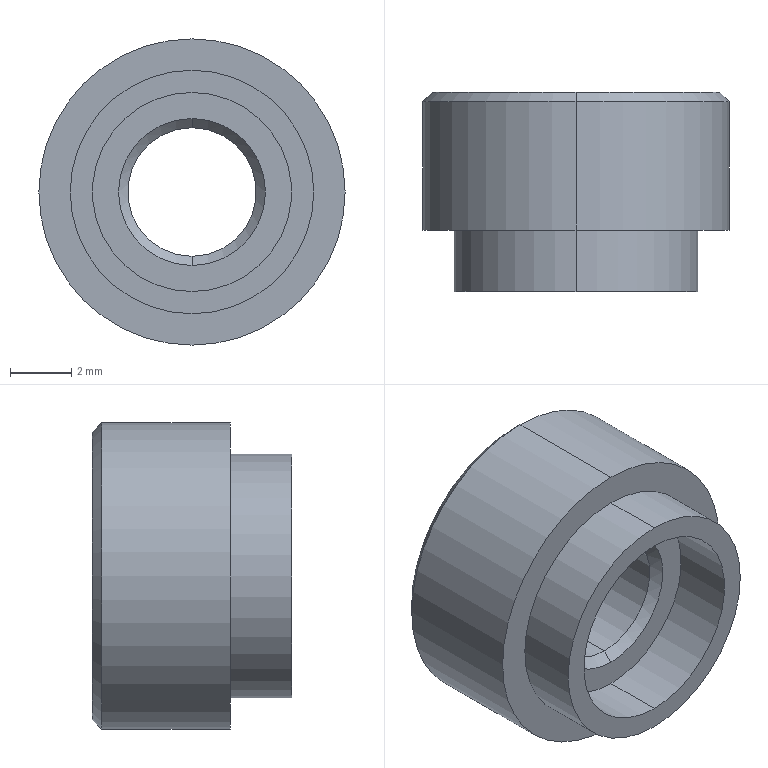Part | SolidWorks | features Chamfer 1, HoleWzd 1, Revolution 1 | 1 solid | 18 faces | box 10 x 6.5 x 10 mm | volume 321.367 mm3 | cylinder 8 | cone 6 | plane 4 | commonest cylinder face diameters 4.2 x2 6.5 x2 7.95 x2 10 x2
STEP:
#1=CARTESIAN_POINT('',(0.,6.5,4.7));
#2=VERTEX_POINT('',#1);
#3=CARTESIAN_POINT('',(0.,6.5,-4.7));
#4=VERTEX_POINT('',#3);
#5=CARTESIAN_POINT('',(0.,6.5,0.));
#6=DIRECTION('',(0.,1.,0.));
#7=DIRECTION('',(0.,0.,-1.));
#8=AXIS2_PLACEMENT_3D('',#5,#6,#7);
#9=CIRCLE('',#8,4.7);
#10=EDGE_CURVE('',#2,#4,#9,.T.);
#11=ORIENTED_EDGE('',*,*,#10,.F.);
#12=CARTESIAN_POINT('',(0.,6.2,5.));
#13=VERTEX_POINT('',#12);
#14=CARTESIAN_POINT('',(0.,6.2,5.));
#15=DIRECTION('',(0.,-0.7071,0.7071));
#16=VECTOR('',#15,1000.);
#17=LINE('',#14,#16);
#18=EDGE_CURVE('',#2,#13,#17,.T.);
#19=ORIENTED_EDGE('',*,*,#18,.T.);
#20=CARTESIAN_POINT('',(0.,6.2,-5.));
#21=VERTEX_POINT('',#20);
#22=CARTESIAN_POINT('',(0.,6.2,0.));
#23=DIRECTION('',(0.,-1.,0.));
#24=DIRECTION('',(0.,0.,-1.));
#25=AXIS2_PLACEMENT_3D('',#22,#23,#24);
#26=CIRCLE('',#25,5.);
#27=EDGE_CURVE('',#21,#13,#26,.T.);
#28=ORIENTED_EDGE('',*,*,#27,.F.);
#29=CARTESIAN_POINT('',(0.,6.2,-5.));
#30=DIRECTION('',(0.,-0.7071,-0.7071));
#31=VECTOR('',#30,1000.);
#32=LINE('',#29,#31);
#33=EDGE_CURVE('',#4,#21,#32,.T.);
#34=ORIENTED_EDGE('',*,*,#33,.F.);
#35=EDGE_LOOP('',(#11,#19,#28,#34));
#36=FACE_OUTER_BOUND('',#35,.T.);
#37=CARTESIAN_POINT('',(0.,6.2,0.));
#38=DIRECTION('',(0.,-1.,0.));
#39=DIRECTION('',(0.,0.,-1.));
#40=AXIS2_PLACEMENT_3D('',#37,#38,#39);
#41=CONICAL_SURFACE('',#40,5.,0.7854);
#42=ADVANCED_FACE('',(#36),#41,.T.);
#43=CARTESIAN_POINT('',(0.,6.2,-2.1));
#44=VERTEX_POINT('',#43);
#45=CARTESIAN_POINT('',(0.,6.2,2.1));
#46=VERTEX_POINT('',#45);
#47=CARTESIAN_POINT('',(0.,6.2,0.));
#48=DIRECTION('',(0.,1.,0.));
#49=DIRECTION('',(0.,0.,-1.));
#50=AXIS2_PLACEMENT_3D('',#47,#48,#49);
#51=CIRCLE('',#50,2.1);
#52=EDGE_CURVE('',#44,#46,#51,.T.);
#53=ORIENTED_EDGE('',*,*,#52,.F.);
#54=CARTESIAN_POINT('',(0.,6.5,-2.4));
#55=VERTEX_POINT('',#54);
#56=CARTESIAN_POINT('',(0.,6.2,-2.1));
#57=DIRECTION('',(0.,0.7071,-0.7071));
#58=VECTOR('',#57,1000.);
#59=LINE('',#56,#58);
#60=EDGE_CURVE('',#44,#55,#59,.T.);
#61=ORIENTED_EDGE('',*,*,#60,.T.);
#62=CARTESIAN_POINT('',(0.,6.5,2.4));
#63=VERTEX_POINT('',#62);
#64=CARTESIAN_POINT('',(0.,6.5,0.));
#65=DIRECTION('',(0.,-1.,0.));
#66=DIRECTION('',(0.,0.,-1.));
#67=AXIS2_PLACEMENT_3D('',#64,#65,#66);
#68=CIRCLE('',#67,2.4);
#69=EDGE_CURVE('',#63,#55,#68,.T.);
#70=ORIENTED_EDGE('',*,*,#69,.F.);
#71=CARTESIAN_POINT('',(0.,6.2,2.1));
#72=DIRECTION('',(0.,0.7071,0.7071));
#73=VECTOR('',#72,1000.);
#74=LINE('',#71,#73);
#75=EDGE_CURVE('',#46,#63,#74,.T.);
#76=ORIENTED_EDGE('',*,*,#75,.F.);
#77=EDGE_LOOP('',(#53,#61,#70,#76));
#78=FACE_OUTER_BOUND('',#77,.T.);
#79=CARTESIAN_POINT('',(0.,6.2,0.));
#80=DIRECTION('',(0.,1.,0.));
#81=DIRECTION('',(0.,0.,1.));
#82=AXIS2_PLACEMENT_3D('',#79,#80,#81);
#83=CONICAL_SURFACE('',#82,2.1,0.7854);
#84=ADVANCED_FACE('',(#78),#83,.F.);
#85=CARTESIAN_POINT('',(0.,2.3,2.1));
#86=VERTEX_POINT('',#85);
#87=CARTESIAN_POINT('',(0.,2.3,-2.1));
#88=VERTEX_POINT('',#87);
#89=CARTESIAN_POINT('',(0.,2.3,0.));
#90=DIRECTION('',(0.,-1.,0.));
#91=DIRECTION('',(0.,0.,1.));
#92=AXIS2_PLACEMENT_3D('',#89,#90,#91);
#93=CIRCLE('',#92,2.1);
#94=EDGE_CURVE('',#86,#88,#93,.T.);
#95=ORIENTED_EDGE('',*,*,#94,.F.);
#96=CARTESIAN_POINT('',(0.,2.,2.4));
#97=VERTEX_POINT('',#96);
#98=CARTESIAN_POINT('',(0.,2.,2.4));
#99=DIRECTION('',(0.,-0.7071,0.7071));
#100=VECTOR('',#99,1000.);
#101=LINE('',#98,#100);
#102=EDGE_CURVE('',#86,#97,#101,.T.);
#103=ORIENTED_EDGE('',*,*,#102,.T.);
#104=CARTESIAN_POINT('',(0.,2.,-2.4));
#105=VERTEX_POINT('',#104);
#106=CARTESIAN_POINT('',(0.,2.,0.));
#107=DIRECTION('',(0.,1.,0.));
#108=DIRECTION('',(0.,0.,1.));
#109=AXIS2_PLACEMENT_3D('',#106,#107,#108);
#110=CIRCLE('',#109,2.4);
#111=EDGE_CURVE('',#105,#97,#110,.T.);
#112=ORIENTED_EDGE('',*,*,#111,.F.);
#113=CARTESIAN_POINT('',(0.,2.,-2.4));
#114=DIRECTION('',(0.,-0.7071,-0.7071));
#115=VECTOR('',#114,1000.);
#116=LINE('',#113,#115);
#117=EDGE_CURVE('',#88,#105,#116,.T.);
#118=ORIENTED_EDGE('',*,*,#117,.F.);
#119=EDGE_LOOP('',(#95,#103,#112,#118));
#120=FACE_OUTER_BOUND('',#119,.T.);
#121=CARTESIAN_POINT('',(0.,2.,0.));
#122=DIRECTION('',(0.,-1.,0.));
#123=DIRECTION('',(0.,0.,-1.));
#124=AXIS2_PLACEMENT_3D('',#121,#122,#123);
#125=CONICAL_SURFACE('',#124,2.4,0.7854);
#126=ADVANCED_FACE('',(#120),#125,.F.);
#127=ORIENTED_EDGE('',*,*,#94,.T.);
#128=CARTESIAN_POINT('',(0.,6.5,-2.1));
#129=DIRECTION('',(0.,1.,0.));
#130=VECTOR('',#129,1000.);
#131=LINE('',#128,#130);
#132=EDGE_CURVE('',#88,#44,#131,.T.);
#133=ORIENTED_EDGE('',*,*,#132,.T.);
#134=ORIENTED_EDGE('',*,*,#52,.T.);
#135=CARTESIAN_POINT('',(0.,6.5,2.1));
#136=DIRECTION('',(0.,1.,0.));
#137=VECTOR('',#136,1000.);
#138=LINE('',#135,#137);
#139=EDGE_CURVE('',#86,#46,#138,.T.);
#140=ORIENTED_EDGE('',*,*,#139,.F.);
#141=EDGE_LOOP('',(#127,#133,#134,#140));
#142=FACE_OUTER_BOUND('',#141,.T.);
#143=CARTESIAN_POINT('',(0.,6.5,0.));
#144=DIRECTION('',(0.,1.,0.));
#145=DIRECTION('',(0.,0.,1.));
#146=AXIS2_PLACEMENT_3D('',#143,#144,#145);
#147=CYLINDRICAL_SURFACE('',#146,2.1);
#148=ADVANCED_FACE('',(#142),#147,.F.);
#149=CARTESIAN_POINT('',(0.,2.,3.25));
#150=VERTEX_POINT('',#149);
#151=CARTESIAN_POINT('',(0.,2.,-3.25));
#152=VERTEX_POINT('',#151);
#153=CARTESIAN_POINT('',(0.,2.,0.));
#154=DIRECTION('',(0.,-1.,0.));
#155=DIRECTION('',(0.,0.,-1.));
#156=AXIS2_PLACEMENT_3D('',#153,#154,#155);
#157=CIRCLE('',#156,3.25);
#158=EDGE_CURVE('',#150,#152,#157,.T.);
#159=ORIENTED_EDGE('',*,*,#158,.F.);
#160=CARTESIAN_POINT('',(0.,0.,3.25));
#161=VERTEX_POINT('',#160);
#162=CARTESIAN_POINT('',(0.,0.,3.25));
#163=DIRECTION('',(0.,-1.,0.));
#164=VECTOR('',#163,1000.);
#165=LINE('',#162,#164);
#166=EDGE_CURVE('',#150,#161,#165,.T.);
#167=ORIENTED_EDGE('',*,*,#166,.T.);
#168=CARTESIAN_POINT('',(0.,0.,-3.25));
#169=VERTEX_POINT('',#168);
#170=CARTESIAN_POINT('',(0.,0.,0.));
#171=DIRECTION('',(0.,-1.,0.));
#172=DIRECTION('',(0.,0.,-1.));
#173=AXIS2_PLACEMENT_3D('',#170,#171,#172);
#174=CIRCLE('',#173,3.25);
#175=EDGE_CURVE('',#161,#169,#174,.T.);
#176=ORIENTED_EDGE('',*,*,#175,.T.);
#177=CARTESIAN_POINT('',(0.,0.,-3.25));
#178=DIRECTION('',(0.,-1.,0.));
#179=VECTOR('',#178,1000.);
#180=LINE('',#177,#179);
#181=EDGE_CURVE('',#152,#169,#180,.T.);
#182=ORIENTED_EDGE('',*,*,#181,.F.);
#183=EDGE_LOOP('',(#159,#167,#176,#182));
#184=FACE_OUTER_BOUND('',#183,.T.);
#185=CARTESIAN_POINT('',(0.,0.,0.));
#186=DIRECTION('',(0.,-1.,0.));
#187=DIRECTION('',(0.,0.,-1.));
#188=AXIS2_PLACEMENT_3D('',#185,#186,#187);
#189=CYLINDRICAL_SURFACE('',#188,3.25);
#190=ADVANCED_FACE('',(#184),#189,.F.);
#191=CARTESIAN_POINT('',(0.,2.,-3.975));
#192=VERTEX_POINT('',#191);
#193=CARTESIAN_POINT('',(0.,2.,3.975));
#194=VERTEX_POINT('',#193);
#195=CARTESIAN_POINT('',(0.,2.,0.));
#196=DIRECTION('',(0.,-1.,0.));
#197=DIRECTION('',(0.,0.,-1.));
#198=AXIS2_PLACEMENT_3D('',#195,#196,#197);
#199=CIRCLE('',#198,3.975);
#200=EDGE_CURVE('',#192,#194,#199,.T.);
#201=ORIENTED_EDGE('',*,*,#200,.T.);
#202=CARTESIAN_POINT('',(0.,0.,3.975));
#203=VERTEX_POINT('',#202);
#204=CARTESIAN_POINT('',(0.,0.,3.975));
#205=DIRECTION('',(0.,-1.,0.));
#206=VECTOR('',#205,1000.);
#207=LINE('',#204,#206);
#208=EDGE_CURVE('',#194,#203,#207,.T.);
#209=ORIENTED_EDGE('',*,*,#208,.T.);
#210=CARTESIAN_POINT('',(0.,0.,-3.975));
#211=VERTEX_POINT('',#210);
#212=CARTESIAN_POINT('',(0.,0.,0.));
#213=DIRECTION('',(0.,-1.,0.));
#214=DIRECTION('',(0.,0.,-1.));
#215=AXIS2_PLACEMENT_3D('',#212,#213,#214);
#216=CIRCLE('',#215,3.975);
#217=EDGE_CURVE('',#211,#203,#216,.T.);
#218=ORIENTED_EDGE('',*,*,#217,.F.);
#219=CARTESIAN_POINT('',(0.,0.,-3.975));
#220=DIRECTION('',(0.,-1.,0.));
#221=VECTOR('',#220,1000.);
#222=LINE('',#219,#221);
#223=EDGE_CURVE('',#192,#211,#222,.T.);
#224=ORIENTED_EDGE('',*,*,#223,.F.);
#225=EDGE_LOOP('',(#201,#209,#218,#224));
#226=FACE_OUTER_BOUND('',#225,.T.);
#227=CARTESIAN_POINT('',(0.,0.,0.));
#228=DIRECTION('',(0.,-1.,0.));
#229=DIRECTION('',(0.,0.,-1.));
#230=AXIS2_PLACEMENT_3D('',#227,#228,#229);
#231=CYLINDRICAL_SURFACE('',#230,3.975);
#232=ADVANCED_FACE('',(#226),#231,.T.);
#233=ORIENTED_EDGE('',*,*,#27,.T.);
#234=CARTESIAN_POINT('',(0.,2.,5.));
#235=VERTEX_POINT('',#234);
#236=CARTESIAN_POINT('',(0.,0.,5.));
#237=DIRECTION('',(0.,-1.,0.));
#238=VECTOR('',#237,1000.);
#239=LINE('',#236,#238);
#240=EDGE_CURVE('',#13,#235,#239,.T.);
#241=ORIENTED_EDGE('',*,*,#240,.T.);
#242=CARTESIAN_POINT('',(0.,2.,-5.));
#243=VERTEX_POINT('',#242);
#244=CARTESIAN_POINT('',(0.,2.,0.));
#245=DIRECTION('',(0.,-1.,0.));
#246=DIRECTION('',(0.,0.,-1.));
#247=AXIS2_PLACEMENT_3D('',#244,#245,#246);
#248=CIRCLE('',#247,5.);
#249=EDGE_CURVE('',#243,#235,#248,.T.);
#250=ORIENTED_EDGE('',*,*,#249,.F.);
#251=CARTESIAN_POINT('',(0.,0.,-5.));
#252=DIRECTION('',(0.,-1.,0.));
#253=VECTOR('',#252,1000.);
#254=LINE('',#251,#253);
#255=EDGE_CURVE('',#21,#243,#254,.T.);
#256=ORIENTED_EDGE('',*,*,#255,.F.);
#257=EDGE_LOOP('',(#233,#241,#250,#256));
#258=FACE_OUTER_BOUND('',#257,.T.);
#259=CARTESIAN_POINT('',(0.,0.,0.));
#260=DIRECTION('',(0.,-1.,0.));
#261=DIRECTION('',(0.,0.,-1.));
#262=AXIS2_PLACEMENT_3D('',#259,#260,#261);
#263=CYLINDRICAL_SURFACE('',#262,5.);
#264=ADVANCED_FACE('',(#258),#263,.T.);
#265=ORIENTED_EDGE('',*,*,#69,.T.);
#266=CARTESIAN_POINT('',(0.,6.5,0.));
#267=DIRECTION('',(0.,-1.,0.));
#268=DIRECTION('',(0.,0.,-1.));
#269=AXIS2_PLACEMENT_3D('',#266,#267,#268);
#270=CIRCLE('',#269,2.4);
#271=EDGE_CURVE('',#55,#63,#270,.T.);
#272=ORIENTED_EDGE('',*,*,#271,.T.);
#273=EDGE_LOOP('',(#265,#272));
#274=FACE_BOUND('',#273,.T.);
#275=CARTESIAN_POINT('',(0.,6.5,0.));
#276=DIRECTION('',(0.,1.,0.));
#277=DIRECTION('',(0.,0.,-1.));
#278=AXIS2_PLACEMENT_3D('',#275,#276,#277);
#279=CIRCLE('',#278,4.7);
#280=EDGE_CURVE('',#4,#2,#279,.T.);
#281=ORIENTED_EDGE('',*,*,#280,.T.);
#282=ORIENTED_EDGE('',*,*,#10,.T.);
#283=EDGE_LOOP('',(#281,#282));
#284=FACE_OUTER_BOUND('',#283,.T.);
#285=CARTESIAN_POINT('',(0.,6.5,0.));
#286=DIRECTION('',(0.,-1.,0.));
#287=DIRECTION('',(0.,0.,-1.));
#288=AXIS2_PLACEMENT_3D('',#285,#286,#287);
#289=PLANE('',#288);
#290=ADVANCED_FACE('',(#274,#284),#289,.F.);
#291=ORIENTED_EDGE('',*,*,#240,.F.);
#292=CARTESIAN_POINT('',(0.,6.2,0.));
#293=DIRECTION('',(0.,-1.,0.));
#294=DIRECTION('',(0.,0.,-1.));
#295=AXIS2_PLACEMENT_3D('',#292,#293,#294);
#296=CIRCLE('',#295,5.);
#297=EDGE_CURVE('',#13,#21,#296,.T.);
#298=ORIENTED_EDGE('',*,*,#297,.T.);
#299=ORIENTED_EDGE('',*,*,#255,.T.);
#300=CARTESIAN_POINT('',(0.,2.,0.));
#301=DIRECTION('',(0.,-1.,0.));
#302=DIRECTION('',(0.,0.,-1.));
#303=AXIS2_PLACEMENT_3D('',#300,#301,#302);
#304=CIRCLE('',#303,5.);
#305=EDGE_CURVE('',#235,#243,#304,.T.);
#306=ORIENTED_EDGE('',*,*,#305,.F.);
#307=EDGE_LOOP('',(#291,#298,#299,#306));
#308=FACE_OUTER_BOUND('',#307,.T.);
#309=CARTESIAN_POINT('',(0.,0.,0.));
#310=DIRECTION('',(0.,-1.,0.));
#311=DIRECTION('',(0.,0.,-1.));
#312=AXIS2_PLACEMENT_3D('',#309,#310,#311);
#313=CYLINDRICAL_SURFACE('',#312,5.);
#314=ADVANCED_FACE('',(#308),#313,.T.);
#315=ORIENTED_EDGE('',*,*,#200,.F.);
#316=CARTESIAN_POINT('',(0.,2.,0.));
#317=DIRECTION('',(0.,-1.,0.));
#318=DIRECTION('',(0.,0.,-1.));
#319=AXIS2_PLACEMENT_3D('',#316,#317,#318);
#320=CIRCLE('',#319,3.975);
#321=EDGE_CURVE('',#194,#192,#320,.T.);
#322=ORIENTED_EDGE('',*,*,#321,.F.);
#323=EDGE_LOOP('',(#315,#322));
#324=FACE_BOUND('',#323,.T.);
#325=ORIENTED_EDGE('',*,*,#249,.T.);
#326=ORIENTED_EDGE('',*,*,#305,.T.);
#327=EDGE_LOOP('',(#325,#326));
#328=FACE_OUTER_BOUND('',#327,.T.);
#329=CARTESIAN_POINT('',(-5.,2.,0.));
#330=DIRECTION('',(0.,1.,0.));
#331=DIRECTION('',(0.,0.,1.));
#332=AXIS2_PLACEMENT_3D('',#329,#330,#331);
#333=PLANE('',#332);
#334=ADVANCED_FACE('',(#324,#328),#333,.F.);
#335=ORIENTED_EDGE('',*,*,#208,.F.);
#336=ORIENTED_EDGE('',*,*,#321,.T.);
#337=ORIENTED_EDGE('',*,*,#223,.T.);
#338=CARTESIAN_POINT('',(0.,0.,0.));
#339=DIRECTION('',(0.,-1.,0.));
#340=DIRECTION('',(0.,0.,-1.));
#341=AXIS2_PLACEMENT_3D('',#338,#339,#340);
#342=CIRCLE('',#341,3.975);
#343=EDGE_CURVE('',#203,#211,#342,.T.);
#344=ORIENTED_EDGE('',*,*,#343,.F.);
#345=EDGE_LOOP('',(#335,#336,#337,#344));
#346=FACE_OUTER_BOUND('',#345,.T.);
#347=CARTESIAN_POINT('',(0.,0.,0.));
#348=DIRECTION('',(0.,-1.,0.));
#349=DIRECTION('',(0.,0.,-1.));
#350=AXIS2_PLACEMENT_3D('',#347,#348,#349);
#351=CYLINDRICAL_SURFACE('',#350,3.975);
#352=ADVANCED_FACE('',(#346),#351,.T.);
#353=CARTESIAN_POINT('',(0.,0.,0.));
#354=DIRECTION('',(0.,-1.,0.));
#355=DIRECTION('',(0.,0.,-1.));
#356=AXIS2_PLACEMENT_3D('',#353,#354,#355);
#357=CIRCLE('',#356,3.25);
#358=EDGE_CURVE('',#169,#161,#357,.T.);
#359=ORIENTED_EDGE('',*,*,#358,.F.);
#360=ORIENTED_EDGE('',*,*,#175,.F.);
#361=EDGE_LOOP('',(#359,#360));
#362=FACE_BOUND('',#361,.T.);
#363=ORIENTED_EDGE('',*,*,#217,.T.);
#364=ORIENTED_EDGE('',*,*,#343,.T.);
#365=EDGE_LOOP('',(#363,#364));
#366=FACE_OUTER_BOUND('',#365,.T.);
#367=CARTESIAN_POINT('',(-3.975,0.,0.));
#368=DIRECTION('',(0.,1.,0.));
#369=DIRECTION('',(0.,0.,1.));
#370=AXIS2_PLACEMENT_3D('',#367,#368,#369);
#371=PLANE('',#370);
#372=ADVANCED_FACE('',(#362,#366),#371,.F.);
#373=ORIENTED_EDGE('',*,*,#166,.F.);
#374=CARTESIAN_POINT('',(0.,2.,0.));
#375=DIRECTION('',(0.,-1.,0.));
#376=DIRECTION('',(0.,0.,-1.));
#377=AXIS2_PLACEMENT_3D('',#374,#375,#376);
#378=CIRCLE('',#377,3.25);
#379=EDGE_CURVE('',#152,#150,#378,.T.);
#380=ORIENTED_EDGE('',*,*,#379,.F.);
#381=ORIENTED_EDGE('',*,*,#181,.T.);
#382=ORIENTED_EDGE('',*,*,#358,.T.);
#383=EDGE_LOOP('',(#373,#380,#381,#382));
#384=FACE_OUTER_BOUND('',#383,.T.);
#385=CARTESIAN_POINT('',(0.,0.,0.));
#386=DIRECTION('',(0.,-1.,0.));
#387=DIRECTION('',(0.,0.,-1.));
#388=AXIS2_PLACEMENT_3D('',#385,#386,#387);
#389=CYLINDRICAL_SURFACE('',#388,3.25);
#390=ADVANCED_FACE('',(#384),#389,.F.);
#391=ORIENTED_EDGE('',*,*,#111,.T.);
#392=CARTESIAN_POINT('',(0.,2.,0.));
#393=DIRECTION('',(0.,1.,0.));
#394=DIRECTION('',(0.,0.,1.));
#395=AXIS2_PLACEMENT_3D('',#392,#393,#394);
#396=CIRCLE('',#395,2.4);
#397=EDGE_CURVE('',#97,#105,#396,.T.);
#398=ORIENTED_EDGE('',*,*,#397,.T.);
#399=EDGE_LOOP('',(#391,#398));
#400=FACE_BOUND('',#399,.T.);
#401=ORIENTED_EDGE('',*,*,#379,.T.);
#402=ORIENTED_EDGE('',*,*,#158,.T.);
#403=EDGE_LOOP('',(#401,#402));
#404=FACE_OUTER_BOUND('',#403,.T.);
#405=CARTESIAN_POINT('',(-3.25,2.,0.));
#406=DIRECTION('',(0.,1.,0.));
#407=DIRECTION('',(0.,0.,1.));
#408=AXIS2_PLACEMENT_3D('',#405,#406,#407);
#409=PLANE('',#408);
#410=ADVANCED_FACE('',(#400,#404),#409,.F.);
#411=ORIENTED_EDGE('',*,*,#132,.F.);
#412=CARTESIAN_POINT('',(0.,2.3,0.));
#413=DIRECTION('',(0.,-1.,0.));
#414=DIRECTION('',(0.,0.,1.));
#415=AXIS2_PLACEMENT_3D('',#412,#413,#414);
#416=CIRCLE('',#415,2.1);
#417=EDGE_CURVE('',#88,#86,#416,.T.);
#418=ORIENTED_EDGE('',*,*,#417,.T.);
#419=ORIENTED_EDGE('',*,*,#139,.T.);
#420=CARTESIAN_POINT('',(0.,6.2,0.));
#421=DIRECTION('',(0.,1.,0.));
#422=DIRECTION('',(0.,0.,-1.));
#423=AXIS2_PLACEMENT_3D('',#420,#421,#422);
#424=CIRCLE('',#423,2.1);
#425=EDGE_CURVE('',#46,#44,#424,.T.);
#426=ORIENTED_EDGE('',*,*,#425,.T.);
#427=EDGE_LOOP('',(#411,#418,#419,#426));
#428=FACE_OUTER_BOUND('',#427,.T.);
#429=CARTESIAN_POINT('',(0.,6.5,0.));
#430=DIRECTION('',(0.,1.,0.));
#431=DIRECTION('',(0.,0.,1.));
#432=AXIS2_PLACEMENT_3D('',#429,#430,#431);
#433=CYLINDRICAL_SURFACE('',#432,2.1);
#434=ADVANCED_FACE('',(#428),#433,.F.);
#435=ORIENTED_EDGE('',*,*,#102,.F.);
#436=ORIENTED_EDGE('',*,*,#417,.F.);
#437=ORIENTED_EDGE('',*,*,#117,.T.);
#438=ORIENTED_EDGE('',*,*,#397,.F.);
#439=EDGE_LOOP('',(#435,#436,#437,#438));
#440=FACE_OUTER_BOUND('',#439,.T.);
#441=CARTESIAN_POINT('',(0.,2.,0.));
#442=DIRECTION('',(0.,-1.,0.));
#443=DIRECTION('',(0.,0.,-1.));
#444=AXIS2_PLACEMENT_3D('',#441,#442,#443);
#445=CONICAL_SURFACE('',#444,2.4,0.7854);
#446=ADVANCED_FACE('',(#440),#445,.F.);
#447=ORIENTED_EDGE('',*,*,#60,.F.);
#448=ORIENTED_EDGE('',*,*,#425,.F.);
#449=ORIENTED_EDGE('',*,*,#75,.T.);
#450=ORIENTED_EDGE('',*,*,#271,.F.);
#451=EDGE_LOOP('',(#447,#448,#449,#450));
#452=FACE_OUTER_BOUND('',#451,.T.);
#453=CARTESIAN_POINT('',(0.,6.2,0.));
#454=DIRECTION('',(0.,1.,0.));
#455=DIRECTION('',(0.,0.,1.));
#456=AXIS2_PLACEMENT_3D('',#453,#454,#455);
#457=CONICAL_SURFACE('',#456,2.1,0.7854);
#458=ADVANCED_FACE('',(#452),#457,.F.);
#459=ORIENTED_EDGE('',*,*,#18,.F.);
#460=ORIENTED_EDGE('',*,*,#280,.F.);
#461=ORIENTED_EDGE('',*,*,#33,.T.);
#462=ORIENTED_EDGE('',*,*,#297,.F.);
#463=EDGE_LOOP('',(#459,#460,#461,#462));
#464=FACE_OUTER_BOUND('',#463,.T.);
#465=CARTESIAN_POINT('',(0.,6.2,0.));
#466=DIRECTION('',(0.,-1.,0.));
#467=DIRECTION('',(0.,0.,-1.));
#468=AXIS2_PLACEMENT_3D('',#465,#466,#467);
#469=CONICAL_SURFACE('',#468,5.,0.7854);
#470=ADVANCED_FACE('',(#464),#469,.T.);
#471=CLOSED_SHELL('',(#42,#84,#126,#148,#190,#232,#264,#290,#314,#334,#352,#372,#390,#410,#434,#446,#458,#470));
#472=MANIFOLD_SOLID_BREP('',#471);
#473=CARTESIAN_POINT('',(0.,0.,0.));
#474=DIRECTION('',(0.,0.,1.));
#475=DIRECTION('',(1.,0.,0.));
#476=AXIS2_PLACEMENT_3D('',#473,#474,#475);
#477=(LENGTH_UNIT()NAMED_UNIT(*)SI_UNIT(.MILLI.,.METRE.));
#478=UNCERTAINTY_MEASURE_WITH_UNIT(LENGTH_MEASURE(0.00001),#477,'','');
#479=(NAMED_UNIT(*)PLANE_ANGLE_UNIT()SI_UNIT($,.RADIAN.));
#480=(NAMED_UNIT(*)SI_UNIT($,.STERADIAN.)SOLID_ANGLE_UNIT());
#481=(GEOMETRIC_REPRESENTATION_CONTEXT(3)GLOBAL_UNCERTAINTY_ASSIGNED_CONTEXT((#478))GLOBAL_UNIT_ASSIGNED_CONTEXT((#477,#479,#480))REPRESENTATION_CONTEXT('',''));
#482=ADVANCED_BREP_SHAPE_REPRESENTATION('',(#472,#476),#481);